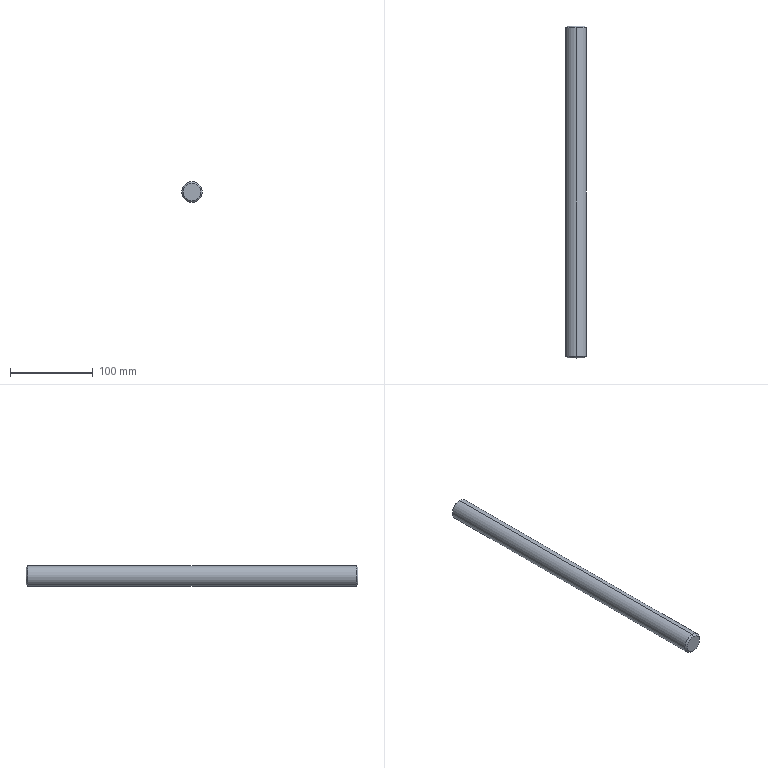Part | STEP file | BCC3 H13_3 | 1 solid | 12 faces | box 25 x 400 x 25 mm | volume 195748 mm3 | cone 6 | cylinder 4 | plane 2 | commonest cylinder face diameters 5 x2 25 x2
STEP:
#1=CARTESIAN_POINT('',(0.,0.,0.));
#2=DIRECTION('',(0.,0.,1.));
#3=DIRECTION('',(1.,0.,0.));
#4=AXIS2_PLACEMENT_3D('',#1,#2,#3);
#5=CARTESIAN_POINT('',(0.,385.,2.5));
#6=VERTEX_POINT('',#5);
#7=CARTESIAN_POINT('',(0.,400.,2.5));
#8=VERTEX_POINT('',#7);
#9=CARTESIAN_POINT('',(0.,400.,2.5));
#10=DIRECTION('',(0.,1.,0.));
#11=VECTOR('',#10,1.);
#12=LINE('',#9,#11);
#13=CARTESIAN_POINT('',(0.,400.,0.));
#14=DIRECTION('',(0.,1.,0.));
#15=DIRECTION('',(0.,0.,1.));
#16=AXIS2_PLACEMENT_3D('',#13,#14,#15);
#17=CYLINDRICAL_SURFACE('',#16,2.5);
#18=CARTESIAN_POINT('',(6.283,0.));
#19=DIRECTION('',(0.,1.));
#20=VECTOR('',#19,1.);
#21=LINE('',#18,#20);
#22=(GEOMETRIC_REPRESENTATION_CONTEXT(2)PARAMETRIC_REPRESENTATION_CONTEXT()REPRESENTATION_CONTEXT('',''));
#23=DEFINITIONAL_REPRESENTATION('',(#21),#22);
#24=PCURVE('',#17,#23);
#25=CARTESIAN_POINT('',(0.,400.,0.));
#26=DIRECTION('',(0.,1.,0.));
#27=DIRECTION('',(0.,0.,1.));
#28=AXIS2_PLACEMENT_3D('',#25,#26,#27);
#29=CYLINDRICAL_SURFACE('',#28,2.5);
#30=CARTESIAN_POINT('',(0.,0.));
#31=DIRECTION('',(0.,1.));
#32=VECTOR('',#31,1.);
#33=LINE('',#30,#32);
#34=(GEOMETRIC_REPRESENTATION_CONTEXT(2)PARAMETRIC_REPRESENTATION_CONTEXT()REPRESENTATION_CONTEXT('',''));
#35=DEFINITIONAL_REPRESENTATION('',(#33),#34);
#36=PCURVE('',#29,#35);
#37=SURFACE_CURVE('',#12,(#24,#36),.PCURVE_S1.);
#38=EDGE_CURVE('',#6,#8,#37,.T.);
#39=ORIENTED_EDGE('',*,*,#38,.T.);
#40=CARTESIAN_POINT('',(0.,400.,-2.5));
#41=VERTEX_POINT('',#40);
#42=CARTESIAN_POINT('',(0.,400.,0.));
#43=DIRECTION('',(0.,1.,0.));
#44=DIRECTION('',(0.,0.,1.));
#45=AXIS2_PLACEMENT_3D('',#42,#43,#44);
#46=CIRCLE('',#45,2.5);
#47=CARTESIAN_POINT('',(0.,0.));
#48=DIRECTION('',(1.,0.));
#49=VECTOR('',#48,1.);
#50=LINE('',#47,#49);
#51=(GEOMETRIC_REPRESENTATION_CONTEXT(2)PARAMETRIC_REPRESENTATION_CONTEXT()REPRESENTATION_CONTEXT('',''));
#52=DEFINITIONAL_REPRESENTATION('',(#50),#51);
#53=PCURVE('',#17,#52);
#54=CARTESIAN_POINT('',(0.,400.,0.));
#55=DIRECTION('',(0.,1.,0.));
#56=DIRECTION('',(0.,0.,1.));
#57=AXIS2_PLACEMENT_3D('',#54,#55,#56);
#58=PLANE('',#57);
#59=CARTESIAN_POINT('',(0.,0.));
#60=DIRECTION('',(1.,0.));
#61=AXIS2_PLACEMENT_2D('',#59,#60);
#62=CIRCLE('',#61,2.5);
#63=(GEOMETRIC_REPRESENTATION_CONTEXT(2)PARAMETRIC_REPRESENTATION_CONTEXT()REPRESENTATION_CONTEXT('',''));
#64=DEFINITIONAL_REPRESENTATION('',(#62),#63);
#65=PCURVE('',#58,#64);
#66=SURFACE_CURVE('',#46,(#53,#65),.PCURVE_S1.);
#67=EDGE_CURVE('',#41,#8,#66,.T.);
#68=ORIENTED_EDGE('',*,*,#67,.F.);
#69=CARTESIAN_POINT('',(0.,385.,-2.5));
#70=VERTEX_POINT('',#69);
#71=CARTESIAN_POINT('',(0.,400.,-2.5));
#72=DIRECTION('',(0.,1.,0.));
#73=VECTOR('',#72,1.);
#74=LINE('',#71,#73);
#75=CARTESIAN_POINT('',(3.142,0.));
#76=DIRECTION('',(0.,1.));
#77=VECTOR('',#76,1.);
#78=LINE('',#75,#77);
#79=(GEOMETRIC_REPRESENTATION_CONTEXT(2)PARAMETRIC_REPRESENTATION_CONTEXT()REPRESENTATION_CONTEXT('',''));
#80=DEFINITIONAL_REPRESENTATION('',(#78),#79);
#81=PCURVE('',#17,#80);
#82=CARTESIAN_POINT('',(3.142,0.));
#83=DIRECTION('',(0.,1.));
#84=VECTOR('',#83,1.);
#85=LINE('',#82,#84);
#86=(GEOMETRIC_REPRESENTATION_CONTEXT(2)PARAMETRIC_REPRESENTATION_CONTEXT()REPRESENTATION_CONTEXT('',''));
#87=DEFINITIONAL_REPRESENTATION('',(#85),#86);
#88=PCURVE('',#29,#87);
#89=SURFACE_CURVE('',#74,(#81,#88),.PCURVE_S1.);
#90=EDGE_CURVE('',#70,#41,#89,.T.);
#91=ORIENTED_EDGE('',*,*,#90,.F.);
#92=CARTESIAN_POINT('',(0.,385.,0.));
#93=DIRECTION('',(0.,1.,0.));
#94=DIRECTION('',(0.,0.,1.));
#95=AXIS2_PLACEMENT_3D('',#92,#93,#94);
#96=CIRCLE('',#95,2.5);
#97=CARTESIAN_POINT('',(0.,-15.));
#98=DIRECTION('',(1.,0.));
#99=VECTOR('',#98,1.);
#100=LINE('',#97,#99);
#101=(GEOMETRIC_REPRESENTATION_CONTEXT(2)PARAMETRIC_REPRESENTATION_CONTEXT()REPRESENTATION_CONTEXT('',''));
#102=DEFINITIONAL_REPRESENTATION('',(#100),#101);
#103=PCURVE('',#17,#102);
#104=CARTESIAN_POINT('',(0.,385.,0.));
#105=DIRECTION('',(0.,1.,0.));
#106=DIRECTION('',(0.,0.,1.));
#107=AXIS2_PLACEMENT_3D('',#104,#105,#106);
#108=CONICAL_SURFACE('',#107,2.5,1.03);
#109=CARTESIAN_POINT('',(0.,0.));
#110=DIRECTION('',(1.,0.));
#111=VECTOR('',#110,1.);
#112=LINE('',#109,#111);
#113=(GEOMETRIC_REPRESENTATION_CONTEXT(2)PARAMETRIC_REPRESENTATION_CONTEXT()REPRESENTATION_CONTEXT('',''));
#114=DEFINITIONAL_REPRESENTATION('',(#112),#113);
#115=PCURVE('',#108,#114);
#116=SURFACE_CURVE('',#96,(#103,#115),.PCURVE_S1.);
#117=EDGE_CURVE('',#70,#6,#116,.T.);
#118=ORIENTED_EDGE('',*,*,#117,.T.);
#119=EDGE_LOOP('',(#39,#68,#91,#118));
#120=FACE_BOUND('',#119,.F.);
#121=ADVANCED_FACE('',(#120),#17,.F.);
#122=ORIENTED_EDGE('',*,*,#117,.F.);
#123=CARTESIAN_POINT('',(0.,383.498,0.));
#124=VERTEX_POINT('',#123);
#125=CARTESIAN_POINT('',(0.,385.,-2.5));
#126=DIRECTION('',(0.,0.515,-0.8572));
#127=VECTOR('',#126,1.);
#128=LINE('',#125,#127);
#129=CARTESIAN_POINT('',(3.142,0.));
#130=DIRECTION('',(0.,1.));
#131=VECTOR('',#130,1.);
#132=LINE('',#129,#131);
#133=(GEOMETRIC_REPRESENTATION_CONTEXT(2)PARAMETRIC_REPRESENTATION_CONTEXT()REPRESENTATION_CONTEXT('',''));
#134=DEFINITIONAL_REPRESENTATION('',(#132),#133);
#135=PCURVE('',#108,#134);
#136=CARTESIAN_POINT('',(0.,385.,0.));
#137=DIRECTION('',(0.,1.,0.));
#138=DIRECTION('',(0.,0.,1.));
#139=AXIS2_PLACEMENT_3D('',#136,#137,#138);
#140=CONICAL_SURFACE('',#139,2.5,1.03);
#141=CARTESIAN_POINT('',(3.142,0.));
#142=DIRECTION('',(0.,1.));
#143=VECTOR('',#142,1.);
#144=LINE('',#141,#143);
#145=(GEOMETRIC_REPRESENTATION_CONTEXT(2)PARAMETRIC_REPRESENTATION_CONTEXT()REPRESENTATION_CONTEXT('',''));
#146=DEFINITIONAL_REPRESENTATION('',(#144),#145);
#147=PCURVE('',#140,#146);
#148=SURFACE_CURVE('',#128,(#135,#147),.PCURVE_S1.);
#149=EDGE_CURVE('',#124,#70,#148,.T.);
#150=ORIENTED_EDGE('',*,*,#149,.F.);
#151=CARTESIAN_POINT('',(0.,385.,2.5));
#152=DIRECTION('',(0.,0.515,0.8572));
#153=VECTOR('',#152,1.);
#154=LINE('',#151,#153);
#155=CARTESIAN_POINT('',(6.283,0.));
#156=DIRECTION('',(0.,1.));
#157=VECTOR('',#156,1.);
#158=LINE('',#155,#157);
#159=(GEOMETRIC_REPRESENTATION_CONTEXT(2)PARAMETRIC_REPRESENTATION_CONTEXT()REPRESENTATION_CONTEXT('',''));
#160=DEFINITIONAL_REPRESENTATION('',(#158),#159);
#161=PCURVE('',#108,#160);
#162=CARTESIAN_POINT('',(0.,0.));
#163=DIRECTION('',(0.,1.));
#164=VECTOR('',#163,1.);
#165=LINE('',#162,#164);
#166=(GEOMETRIC_REPRESENTATION_CONTEXT(2)PARAMETRIC_REPRESENTATION_CONTEXT()REPRESENTATION_CONTEXT('',''));
#167=DEFINITIONAL_REPRESENTATION('',(#165),#166);
#168=PCURVE('',#140,#167);
#169=SURFACE_CURVE('',#154,(#161,#168),.PCURVE_S1.);
#170=EDGE_CURVE('',#124,#6,#169,.T.);
#171=ORIENTED_EDGE('',*,*,#170,.T.);
#172=EDGE_LOOP('',(#122,#150,#171));
#173=FACE_BOUND('',#172,.F.);
#174=ADVANCED_FACE('',(#173),#108,.F.);
#175=CARTESIAN_POINT('',(0.,400.,10.5));
#176=VERTEX_POINT('',#175);
#177=CARTESIAN_POINT('',(0.,400.,-10.5));
#178=VERTEX_POINT('',#177);
#179=CARTESIAN_POINT('',(0.,400.,0.));
#180=DIRECTION('',(0.,1.,0.));
#181=DIRECTION('',(0.,0.,1.));
#182=AXIS2_PLACEMENT_3D('',#179,#180,#181);
#183=CIRCLE('',#182,10.5);
#184=CARTESIAN_POINT('',(0.,400.,0.));
#185=DIRECTION('',(0.,-1.,0.));
#186=DIRECTION('',(0.,0.,-1.));
#187=AXIS2_PLACEMENT_3D('',#184,#185,#186);
#188=CONICAL_SURFACE('',#187,10.5,0.7854);
#189=CARTESIAN_POINT('',(3.142,0.));
#190=DIRECTION('',(-1.,0.));
#191=VECTOR('',#190,1.);
#192=LINE('',#189,#191);
#193=(GEOMETRIC_REPRESENTATION_CONTEXT(2)PARAMETRIC_REPRESENTATION_CONTEXT()REPRESENTATION_CONTEXT('',''));
#194=DEFINITIONAL_REPRESENTATION('',(#192),#193);
#195=PCURVE('',#188,#194);
#196=CARTESIAN_POINT('',(0.,0.));
#197=DIRECTION('',(1.,0.));
#198=AXIS2_PLACEMENT_2D('',#196,#197);
#199=CIRCLE('',#198,10.5);
#200=(GEOMETRIC_REPRESENTATION_CONTEXT(2)PARAMETRIC_REPRESENTATION_CONTEXT()REPRESENTATION_CONTEXT('',''));
#201=DEFINITIONAL_REPRESENTATION('',(#199),#200);
#202=PCURVE('',#58,#201);
#203=SURFACE_CURVE('',#183,(#195,#202),.PCURVE_S1.);
#204=EDGE_CURVE('',#176,#178,#203,.T.);
#205=ORIENTED_EDGE('',*,*,#204,.F.);
#206=CARTESIAN_POINT('',(0.,398.,12.5));
#207=VERTEX_POINT('',#206);
#208=CARTESIAN_POINT('',(0.,400.,10.5));
#209=DIRECTION('',(0.,-0.7071,0.7071));
#210=VECTOR('',#209,1.);
#211=LINE('',#208,#210);
#212=CARTESIAN_POINT('',(3.142,0.));
#213=DIRECTION('',(0.,1.));
#214=VECTOR('',#213,1.);
#215=LINE('',#212,#214);
#216=(GEOMETRIC_REPRESENTATION_CONTEXT(2)PARAMETRIC_REPRESENTATION_CONTEXT()REPRESENTATION_CONTEXT('',''));
#217=DEFINITIONAL_REPRESENTATION('',(#215),#216);
#218=PCURVE('',#188,#217);
#219=CARTESIAN_POINT('',(0.,400.,0.));
#220=DIRECTION('',(0.,-1.,0.));
#221=DIRECTION('',(0.,0.,-1.));
#222=AXIS2_PLACEMENT_3D('',#219,#220,#221);
#223=CONICAL_SURFACE('',#222,10.5,0.7854);
#224=CARTESIAN_POINT('',(3.142,0.));
#225=DIRECTION('',(0.,1.));
#226=VECTOR('',#225,1.);
#227=LINE('',#224,#226);
#228=(GEOMETRIC_REPRESENTATION_CONTEXT(2)PARAMETRIC_REPRESENTATION_CONTEXT()REPRESENTATION_CONTEXT('',''));
#229=DEFINITIONAL_REPRESENTATION('',(#227),#228);
#230=PCURVE('',#223,#229);
#231=SURFACE_CURVE('',#211,(#218,#230),.PCURVE_S1.);
#232=EDGE_CURVE('',#176,#207,#231,.T.);
#233=ORIENTED_EDGE('',*,*,#232,.T.);
#234=CARTESIAN_POINT('',(0.,398.,-12.5));
#235=VERTEX_POINT('',#234);
#236=CARTESIAN_POINT('',(0.,398.,0.));
#237=DIRECTION('',(0.,-1.,0.));
#238=DIRECTION('',(0.,0.,1.));
#239=AXIS2_PLACEMENT_3D('',#236,#237,#238);
#240=CIRCLE('',#239,12.5);
#241=CARTESIAN_POINT('',(-3.142,2.));
#242=DIRECTION('',(1.,0.));
#243=VECTOR('',#242,1.);
#244=LINE('',#241,#243);
#245=(GEOMETRIC_REPRESENTATION_CONTEXT(2)PARAMETRIC_REPRESENTATION_CONTEXT()REPRESENTATION_CONTEXT('',''));
#246=DEFINITIONAL_REPRESENTATION('',(#244),#245);
#247=PCURVE('',#188,#246);
#248=CARTESIAN_POINT('',(0.,400.,0.));
#249=DIRECTION('',(0.,-1.,0.));
#250=DIRECTION('',(0.,0.,-1.));
#251=AXIS2_PLACEMENT_3D('',#248,#249,#250);
#252=CYLINDRICAL_SURFACE('',#251,12.5);
#253=CARTESIAN_POINT('',(-3.142,2.));
#254=DIRECTION('',(1.,0.));
#255=VECTOR('',#254,1.);
#256=LINE('',#253,#255);
#257=(GEOMETRIC_REPRESENTATION_CONTEXT(2)PARAMETRIC_REPRESENTATION_CONTEXT()REPRESENTATION_CONTEXT('',''));
#258=DEFINITIONAL_REPRESENTATION('',(#256),#257);
#259=PCURVE('',#252,#258);
#260=SURFACE_CURVE('',#240,(#247,#259),.PCURVE_S1.);
#261=EDGE_CURVE('',#235,#207,#260,.T.);
#262=ORIENTED_EDGE('',*,*,#261,.F.);
#263=CARTESIAN_POINT('',(0.,400.,-10.5));
#264=DIRECTION('',(0.,-0.7071,-0.7071));
#265=VECTOR('',#264,1.);
#266=LINE('',#263,#265);
#267=CARTESIAN_POINT('',(0.,0.));
#268=DIRECTION('',(0.,1.));
#269=VECTOR('',#268,1.);
#270=LINE('',#267,#269);
#271=(GEOMETRIC_REPRESENTATION_CONTEXT(2)PARAMETRIC_REPRESENTATION_CONTEXT()REPRESENTATION_CONTEXT('',''));
#272=DEFINITIONAL_REPRESENTATION('',(#270),#271);
#273=PCURVE('',#188,#272);
#274=CARTESIAN_POINT('',(6.283,0.));
#275=DIRECTION('',(0.,1.));
#276=VECTOR('',#275,1.);
#277=LINE('',#274,#276);
#278=(GEOMETRIC_REPRESENTATION_CONTEXT(2)PARAMETRIC_REPRESENTATION_CONTEXT()REPRESENTATION_CONTEXT('',''));
#279=DEFINITIONAL_REPRESENTATION('',(#277),#278);
#280=PCURVE('',#223,#279);
#281=SURFACE_CURVE('',#266,(#273,#280),.PCURVE_S1.);
#282=EDGE_CURVE('',#178,#235,#281,.T.);
#283=ORIENTED_EDGE('',*,*,#282,.F.);
#284=EDGE_LOOP('',(#205,#233,#262,#283));
#285=FACE_BOUND('',#284,.T.);
#286=ADVANCED_FACE('',(#285),#188,.T.);
#287=CARTESIAN_POINT('',(0.,0.,-10.5));
#288=VERTEX_POINT('',#287);
#289=CARTESIAN_POINT('',(0.,0.,10.5));
#290=VERTEX_POINT('',#289);
#291=CARTESIAN_POINT('',(0.,0.,0.));
#292=DIRECTION('',(0.,-1.,0.));
#293=DIRECTION('',(0.,0.,1.));
#294=AXIS2_PLACEMENT_3D('',#291,#292,#293);
#295=CIRCLE('',#294,10.5);
#296=CARTESIAN_POINT('',(0.,2.,0.));
#297=DIRECTION('',(0.,1.,0.));
#298=DIRECTION('',(0.,0.,1.));
#299=AXIS2_PLACEMENT_3D('',#296,#297,#298);
#300=CONICAL_SURFACE('',#299,12.5,0.7854);
#301=CARTESIAN_POINT('',(6.283,-2.));
#302=DIRECTION('',(-1.,0.));
#303=VECTOR('',#302,1.);
#304=LINE('',#301,#303);
#305=(GEOMETRIC_REPRESENTATION_CONTEXT(2)PARAMETRIC_REPRESENTATION_CONTEXT()REPRESENTATION_CONTEXT('',''));
#306=DEFINITIONAL_REPRESENTATION('',(#304),#305);
#307=PCURVE('',#300,#306);
#308=CARTESIAN_POINT('',(0.,0.,0.));
#309=DIRECTION('',(0.,1.,0.));
#310=DIRECTION('',(0.,0.,1.));
#311=AXIS2_PLACEMENT_3D('',#308,#309,#310);
#312=PLANE('',#311);
#313=CARTESIAN_POINT('',(10.5,0.));
#314=CARTESIAN_POINT('',(10.5,-18.187));
#315=CARTESIAN_POINT('',(-5.25,-9.093));
#316=CARTESIAN_POINT('',(-21.,0.));
#317=CARTESIAN_POINT('',(-5.25,9.093));
#318=CARTESIAN_POINT('',(10.5,18.187));
#319=CARTESIAN_POINT('',(10.5,0.));
#320=(BOUNDED_CURVE()B_SPLINE_CURVE(2,(#313,#314,#315,#316,#317,#318,#319),.UNSPECIFIED.,.T.,.F.)B_SPLINE_CURVE_WITH_KNOTS((1,2,2,2,2,1),(-2.094,0.,2.094,4.189,6.283,8.378),.UNSPECIFIED.)CURVE()GEOMETRIC_REPRESENTATION_ITEM()RATIONAL_B_SPLINE_CURVE((1.,0.5,1.,0.5,1.,0.5,1.))REPRESENTATION_ITEM(''));
#321=(GEOMETRIC_REPRESENTATION_CONTEXT(2)PARAMETRIC_REPRESENTATION_CONTEXT()REPRESENTATION_CONTEXT('',''));
#322=DEFINITIONAL_REPRESENTATION('',(#320),#321);
#323=PCURVE('',#312,#322);
#324=SURFACE_CURVE('',#295,(#307,#323),.PCURVE_S1.);
#325=EDGE_CURVE('',#288,#290,#324,.T.);
#326=ORIENTED_EDGE('',*,*,#325,.F.);
#327=CARTESIAN_POINT('',(0.,2.,-12.5));
#328=VERTEX_POINT('',#327);
#329=CARTESIAN_POINT('',(0.,2.,-12.5));
#330=DIRECTION('',(0.,0.7071,-0.7071));
#331=VECTOR('',#330,1.);
#332=LINE('',#329,#331);
#333=CARTESIAN_POINT('',(3.142,0.));
#334=DIRECTION('',(0.,1.));
#335=VECTOR('',#334,1.);
#336=LINE('',#333,#335);
#337=(GEOMETRIC_REPRESENTATION_CONTEXT(2)PARAMETRIC_REPRESENTATION_CONTEXT()REPRESENTATION_CONTEXT('',''));
#338=DEFINITIONAL_REPRESENTATION('',(#336),#337);
#339=PCURVE('',#300,#338);
#340=CARTESIAN_POINT('',(0.,2.,0.));
#341=DIRECTION('',(0.,1.,0.));
#342=DIRECTION('',(0.,0.,1.));
#343=AXIS2_PLACEMENT_3D('',#340,#341,#342);
#344=CONICAL_SURFACE('',#343,12.5,0.7854);
#345=CARTESIAN_POINT('',(3.142,0.));
#346=DIRECTION('',(0.,1.));
#347=VECTOR('',#346,1.);
#348=LINE('',#345,#347);
#349=(GEOMETRIC_REPRESENTATION_CONTEXT(2)PARAMETRIC_REPRESENTATION_CONTEXT()REPRESENTATION_CONTEXT('',''));
#350=DEFINITIONAL_REPRESENTATION('',(#348),#349);
#351=PCURVE('',#344,#350);
#352=SURFACE_CURVE('',#332,(#339,#351),.PCURVE_S1.);
#353=EDGE_CURVE('',#288,#328,#352,.T.);
#354=ORIENTED_EDGE('',*,*,#353,.T.);
#355=CARTESIAN_POINT('',(0.,2.,12.5));
#356=VERTEX_POINT('',#355);
#357=CARTESIAN_POINT('',(0.,2.,0.));
#358=DIRECTION('',(0.,1.,0.));
#359=DIRECTION('',(0.,0.,1.));
#360=AXIS2_PLACEMENT_3D('',#357,#358,#359);
#361=CIRCLE('',#360,12.5);
#362=CARTESIAN_POINT('',(0.,0.));
#363=DIRECTION('',(1.,0.));
#364=VECTOR('',#363,1.);
#365=LINE('',#362,#364);
#366=(GEOMETRIC_REPRESENTATION_CONTEXT(2)PARAMETRIC_REPRESENTATION_CONTEXT()REPRESENTATION_CONTEXT('',''));
#367=DEFINITIONAL_REPRESENTATION('',(#365),#366);
#368=PCURVE('',#300,#367);
#369=CARTESIAN_POINT('',(3.142,398.));
#370=DIRECTION('',(-1.,0.));
#371=VECTOR('',#370,1.);
#372=LINE('',#369,#371);
#373=(GEOMETRIC_REPRESENTATION_CONTEXT(2)PARAMETRIC_REPRESENTATION_CONTEXT()REPRESENTATION_CONTEXT('',''));
#374=DEFINITIONAL_REPRESENTATION('',(#372),#373);
#375=PCURVE('',#252,#374);
#376=SURFACE_CURVE('',#361,(#368,#375),.PCURVE_S1.);
#377=EDGE_CURVE('',#356,#328,#376,.T.);
#378=ORIENTED_EDGE('',*,*,#377,.F.);
#379=CARTESIAN_POINT('',(0.,2.,12.5));
#380=DIRECTION('',(0.,0.7071,0.7071));
#381=VECTOR('',#380,1.);
#382=LINE('',#379,#381);
#383=CARTESIAN_POINT('',(0.,0.));
#384=DIRECTION('',(0.,1.));
#385=VECTOR('',#384,1.);
#386=LINE('',#383,#385);
#387=(GEOMETRIC_REPRESENTATION_CONTEXT(2)PARAMETRIC_REPRESENTATION_CONTEXT()REPRESENTATION_CONTEXT('',''));
#388=DEFINITIONAL_REPRESENTATION('',(#386),#387);
#389=PCURVE('',#300,#388);
#390=CARTESIAN_POINT('',(6.283,0.));
#391=DIRECTION('',(0.,1.));
#392=VECTOR('',#391,1.);
#393=LINE('',#390,#392);
#394=(GEOMETRIC_REPRESENTATION_CONTEXT(2)PARAMETRIC_REPRESENTATION_CONTEXT()REPRESENTATION_CONTEXT('',''));
#395=DEFINITIONAL_REPRESENTATION('',(#393),#394);
#396=PCURVE('',#344,#395);
#397=SURFACE_CURVE('',#382,(#389,#396),.PCURVE_S1.);
#398=EDGE_CURVE('',#290,#356,#397,.T.);
#399=ORIENTED_EDGE('',*,*,#398,.F.);
#400=EDGE_LOOP('',(#326,#354,#378,#399));
#401=FACE_BOUND('',#400,.T.);
#402=ADVANCED_FACE('',(#401),#300,.T.);
#403=ORIENTED_EDGE('',*,*,#261,.T.);
#404=CARTESIAN_POINT('',(0.,400.,12.5));
#405=DIRECTION('',(0.,-1.,0.));
#406=VECTOR('',#405,1.);
#407=LINE('',#404,#406);
#408=CARTESIAN_POINT('',(3.142,0.));
#409=DIRECTION('',(0.,1.));
#410=VECTOR('',#409,1.);
#411=LINE('',#408,#410);
#412=(GEOMETRIC_REPRESENTATION_CONTEXT(2)PARAMETRIC_REPRESENTATION_CONTEXT()REPRESENTATION_CONTEXT('',''));
#413=DEFINITIONAL_REPRESENTATION('',(#411),#412);
#414=PCURVE('',#252,#413);
#415=CARTESIAN_POINT('',(0.,400.,0.));
#416=DIRECTION('',(0.,-1.,0.));
#417=DIRECTION('',(0.,0.,-1.));
#418=AXIS2_PLACEMENT_3D('',#415,#416,#417);
#419=CYLINDRICAL_SURFACE('',#418,12.5);
#420=CARTESIAN_POINT('',(3.142,0.));
#421=DIRECTION('',(0.,1.));
#422=VECTOR('',#421,1.);
#423=LINE('',#420,#422);
#424=(GEOMETRIC_REPRESENTATION_CONTEXT(2)PARAMETRIC_REPRESENTATION_CONTEXT()REPRESENTATION_CONTEXT('',''));
#425=DEFINITIONAL_REPRESENTATION('',(#423),#424);
#426=PCURVE('',#419,#425);
#427=SURFACE_CURVE('',#407,(#414,#426),.PCURVE_S1.);
#428=EDGE_CURVE('',#207,#356,#427,.T.);
#429=ORIENTED_EDGE('',*,*,#428,.T.);
#430=ORIENTED_EDGE('',*,*,#377,.T.);
#431=CARTESIAN_POINT('',(0.,400.,-12.5));
#432=DIRECTION('',(0.,-1.,0.));
#433=VECTOR('',#432,1.);
#434=LINE('',#431,#433);
#435=CARTESIAN_POINT('',(0.,0.));
#436=DIRECTION('',(0.,1.));
#437=VECTOR('',#436,1.);
#438=LINE('',#435,#437);
#439=(GEOMETRIC_REPRESENTATION_CONTEXT(2)PARAMETRIC_REPRESENTATION_CONTEXT()REPRESENTATION_CONTEXT('',''));
#440=DEFINITIONAL_REPRESENTATION('',(#438),#439);
#441=PCURVE('',#252,#440);
#442=CARTESIAN_POINT('',(6.283,0.));
#443=DIRECTION('',(0.,1.));
#444=VECTOR('',#443,1.);
#445=LINE('',#442,#444);
#446=(GEOMETRIC_REPRESENTATION_CONTEXT(2)PARAMETRIC_REPRESENTATION_CONTEXT()REPRESENTATION_CONTEXT('',''));
#447=DEFINITIONAL_REPRESENTATION('',(#445),#446);
#448=PCURVE('',#419,#447);
#449=SURFACE_CURVE('',#434,(#441,#448),.PCURVE_S1.);
#450=EDGE_CURVE('',#235,#328,#449,.T.);
#451=ORIENTED_EDGE('',*,*,#450,.F.);
#452=EDGE_LOOP('',(#403,#429,#430,#451));
#453=FACE_BOUND('',#452,.T.);
#454=ADVANCED_FACE('',(#453),#252,.T.);
#455=ORIENTED_EDGE('',*,*,#428,.F.);
#456=CARTESIAN_POINT('',(0.,398.,0.));
#457=DIRECTION('',(0.,-1.,0.));
#458=DIRECTION('',(0.,0.,1.));
#459=AXIS2_PLACEMENT_3D('',#456,#457,#458);
#460=CIRCLE('',#459,12.5);
#461=CARTESIAN_POINT('',(3.142,2.));
#462=DIRECTION('',(1.,0.));
#463=VECTOR('',#462,1.);
#464=LINE('',#461,#463);
#465=(GEOMETRIC_REPRESENTATION_CONTEXT(2)PARAMETRIC_REPRESENTATION_CONTEXT()REPRESENTATION_CONTEXT('',''));
#466=DEFINITIONAL_REPRESENTATION('',(#464),#465);
#467=PCURVE('',#419,#466);
#468=CARTESIAN_POINT('',(3.142,2.));
#469=DIRECTION('',(1.,0.));
#470=VECTOR('',#469,1.);
#471=LINE('',#468,#470);
#472=(GEOMETRIC_REPRESENTATION_CONTEXT(2)PARAMETRIC_REPRESENTATION_CONTEXT()REPRESENTATION_CONTEXT('',''));
#473=DEFINITIONAL_REPRESENTATION('',(#471),#472);
#474=PCURVE('',#223,#473);
#475=SURFACE_CURVE('',#460,(#467,#474),.PCURVE_S1.);
#476=EDGE_CURVE('',#207,#235,#475,.T.);
#477=ORIENTED_EDGE('',*,*,#476,.T.);
#478=ORIENTED_EDGE('',*,*,#450,.T.);
#479=CARTESIAN_POINT('',(0.,2.,0.));
#480=DIRECTION('',(0.,1.,0.));
#481=DIRECTION('',(0.,0.,1.));
#482=AXIS2_PLACEMENT_3D('',#479,#480,#481);
#483=CIRCLE('',#482,12.5);
#484=CARTESIAN_POINT('',(9.425,398.));
#485=DIRECTION('',(-1.,0.));
#486=VECTOR('',#485,1.);
#487=LINE('',#484,#486);
#488=(GEOMETRIC_REPRESENTATION_CONTEXT(2)PARAMETRIC_REPRESENTATION_CONTEXT()REPRESENTATION_CONTEXT('',''));
#489=DEFINITIONAL_REPRESENTATION('',(#487),#488);
#490=PCURVE('',#419,#489);
#491=CARTESIAN_POINT('',(0.,0.));
#492=DIRECTION('',(1.,0.));
#493=VECTOR('',#492,1.);
#494=LINE('',#491,#493);
#495=(GEOMETRIC_REPRESENTATION_CONTEXT(2)PARAMETRIC_REPRESENTATION_CONTEXT()REPRESENTATION_CONTEXT('',''));
#496=DEFINITIONAL_REPRESENTATION('',(#494),#495);
#497=PCURVE('',#344,#496);
#498=SURFACE_CURVE('',#483,(#490,#497),.PCURVE_S1.);
#499=EDGE_CURVE('',#328,#356,#498,.T.);
#500=ORIENTED_EDGE('',*,*,#499,.T.);
#501=EDGE_LOOP('',(#455,#477,#478,#500));
#502=FACE_BOUND('',#501,.T.);
#503=ADVANCED_FACE('',(#502),#419,.T.);
#504=CARTESIAN_POINT('',(0.,400.,0.));
#505=DIRECTION('',(0.,1.,0.));
#506=DIRECTION('',(0.,0.,1.));
#507=AXIS2_PLACEMENT_3D('',#504,#505,#506);
#508=CIRCLE('',#507,2.5);
#509=CARTESIAN_POINT('',(0.,0.));
#510=DIRECTION('',(1.,0.));
#511=AXIS2_PLACEMENT_2D('',#509,#510);
#512=CIRCLE('',#511,2.5);
#513=(GEOMETRIC_REPRESENTATION_CONTEXT(2)PARAMETRIC_REPRESENTATION_CONTEXT()REPRESENTATION_CONTEXT('',''));
#514=DEFINITIONAL_REPRESENTATION('',(#512),#513);
#515=PCURVE('',#58,#514);
#516=CARTESIAN_POINT('',(0.,0.));
#517=DIRECTION('',(1.,0.));
#518=VECTOR('',#517,1.);
#519=LINE('',#516,#518);
#520=(GEOMETRIC_REPRESENTATION_CONTEXT(2)PARAMETRIC_REPRESENTATION_CONTEXT()REPRESENTATION_CONTEXT('',''));
#521=DEFINITIONAL_REPRESENTATION('',(#519),#520);
#522=PCURVE('',#29,#521);
#523=SURFACE_CURVE('',#508,(#515,#522),.PCURVE_S1.);
#524=EDGE_CURVE('',#8,#41,#523,.T.);
#525=ORIENTED_EDGE('',*,*,#524,.F.);
#526=ORIENTED_EDGE('',*,*,#67,.F.);
#527=EDGE_LOOP('',(#525,#526));
#528=FACE_BOUND('',#527,.T.);
#529=CARTESIAN_POINT('',(0.,400.,0.));
#530=DIRECTION('',(0.,1.,0.));
#531=DIRECTION('',(0.,0.,1.));
#532=AXIS2_PLACEMENT_3D('',#529,#530,#531);
#533=CIRCLE('',#532,10.5);
#534=CARTESIAN_POINT('',(0.,0.));
#535=DIRECTION('',(1.,0.));
#536=AXIS2_PLACEMENT_2D('',#534,#535);
#537=CIRCLE('',#536,10.5);
#538=(GEOMETRIC_REPRESENTATION_CONTEXT(2)PARAMETRIC_REPRESENTATION_CONTEXT()REPRESENTATION_CONTEXT('',''));
#539=DEFINITIONAL_REPRESENTATION('',(#537),#538);
#540=PCURVE('',#58,#539);
#541=CARTESIAN_POINT('',(9.425,0.));
#542=DIRECTION('',(-1.,0.));
#543=VECTOR('',#542,1.);
#544=LINE('',#541,#543);
#545=(GEOMETRIC_REPRESENTATION_CONTEXT(2)PARAMETRIC_REPRESENTATION_CONTEXT()REPRESENTATION_CONTEXT('',''));
#546=DEFINITIONAL_REPRESENTATION('',(#544),#545);
#547=PCURVE('',#223,#546);
#548=SURFACE_CURVE('',#533,(#540,#547),.PCURVE_S1.);
#549=EDGE_CURVE('',#178,#176,#548,.T.);
#550=ORIENTED_EDGE('',*,*,#549,.T.);
#551=ORIENTED_EDGE('',*,*,#204,.T.);
#552=EDGE_LOOP('',(#550,#551));
#553=FACE_BOUND('',#552,.T.);
#554=ADVANCED_FACE('',(#528,#553),#58,.T.);
#555=CARTESIAN_POINT('',(0.,0.,0.));
#556=DIRECTION('',(0.,-1.,0.));
#557=DIRECTION('',(0.,0.,1.));
#558=AXIS2_PLACEMENT_3D('',#555,#556,#557);
#559=CIRCLE('',#558,10.5);
#560=CARTESIAN_POINT('',(10.5,0.));
#561=CARTESIAN_POINT('',(10.5,-18.187));
#562=CARTESIAN_POINT('',(-5.25,-9.093));
#563=CARTESIAN_POINT('',(-21.,0.));
#564=CARTESIAN_POINT('',(-5.25,9.093));
#565=CARTESIAN_POINT('',(10.5,18.187));
#566=CARTESIAN_POINT('',(10.5,0.));
#567=(BOUNDED_CURVE()B_SPLINE_CURVE(2,(#560,#561,#562,#563,#564,#565,#566),.UNSPECIFIED.,.T.,.F.)B_SPLINE_CURVE_WITH_KNOTS((1,2,2,2,2,1),(-2.094,0.,2.094,4.189,6.283,8.378),.UNSPECIFIED.)CURVE()GEOMETRIC_REPRESENTATION_ITEM()RATIONAL_B_SPLINE_CURVE((1.,0.5,1.,0.5,1.,0.5,1.))REPRESENTATION_ITEM(''));
#568=(GEOMETRIC_REPRESENTATION_CONTEXT(2)PARAMETRIC_REPRESENTATION_CONTEXT()REPRESENTATION_CONTEXT('',''));
#569=DEFINITIONAL_REPRESENTATION('',(#567),#568);
#570=PCURVE('',#312,#569);
#571=CARTESIAN_POINT('',(6.283,-2.));
#572=DIRECTION('',(-1.,0.));
#573=VECTOR('',#572,1.);
#574=LINE('',#571,#573);
#575=(GEOMETRIC_REPRESENTATION_CONTEXT(2)PARAMETRIC_REPRESENTATION_CONTEXT()REPRESENTATION_CONTEXT('',''));
#576=DEFINITIONAL_REPRESENTATION('',(#574),#575);
#577=PCURVE('',#344,#576);
#578=SURFACE_CURVE('',#559,(#570,#577),.PCURVE_S1.);
#579=EDGE_CURVE('',#290,#288,#578,.T.);
#580=ORIENTED_EDGE('',*,*,#579,.T.);
#581=ORIENTED_EDGE('',*,*,#325,.T.);
#582=EDGE_LOOP('',(#580,#581));
#583=FACE_BOUND('',#582,.T.);
#584=ADVANCED_FACE('',(#583),#312,.F.);
#585=ORIENTED_EDGE('',*,*,#353,.F.);
#586=ORIENTED_EDGE('',*,*,#579,.F.);
#587=ORIENTED_EDGE('',*,*,#398,.T.);
#588=ORIENTED_EDGE('',*,*,#499,.F.);
#589=EDGE_LOOP('',(#585,#586,#587,#588));
#590=FACE_BOUND('',#589,.T.);
#591=ADVANCED_FACE('',(#590),#344,.T.);
#592=ORIENTED_EDGE('',*,*,#232,.F.);
#593=ORIENTED_EDGE('',*,*,#549,.F.);
#594=ORIENTED_EDGE('',*,*,#282,.T.);
#595=ORIENTED_EDGE('',*,*,#476,.F.);
#596=EDGE_LOOP('',(#592,#593,#594,#595));
#597=FACE_BOUND('',#596,.T.);
#598=ADVANCED_FACE('',(#597),#223,.T.);
#599=CARTESIAN_POINT('',(0.,385.,0.));
#600=DIRECTION('',(0.,1.,0.));
#601=DIRECTION('',(0.,0.,1.));
#602=AXIS2_PLACEMENT_3D('',#599,#600,#601);
#603=CIRCLE('',#602,2.5);
#604=CARTESIAN_POINT('',(0.,0.));
#605=DIRECTION('',(1.,0.));
#606=VECTOR('',#605,1.);
#607=LINE('',#604,#606);
#608=(GEOMETRIC_REPRESENTATION_CONTEXT(2)PARAMETRIC_REPRESENTATION_CONTEXT()REPRESENTATION_CONTEXT('',''));
#609=DEFINITIONAL_REPRESENTATION('',(#607),#608);
#610=PCURVE('',#140,#609);
#611=CARTESIAN_POINT('',(0.,-15.));
#612=DIRECTION('',(1.,0.));
#613=VECTOR('',#612,1.);
#614=LINE('',#611,#613);
#615=(GEOMETRIC_REPRESENTATION_CONTEXT(2)PARAMETRIC_REPRESENTATION_CONTEXT()REPRESENTATION_CONTEXT('',''));
#616=DEFINITIONAL_REPRESENTATION('',(#614),#615);
#617=PCURVE('',#29,#616);
#618=SURFACE_CURVE('',#603,(#610,#617),.PCURVE_S1.);
#619=EDGE_CURVE('',#6,#70,#618,.T.);
#620=ORIENTED_EDGE('',*,*,#619,.F.);
#621=ORIENTED_EDGE('',*,*,#170,.F.);
#622=ORIENTED_EDGE('',*,*,#149,.T.);
#623=EDGE_LOOP('',(#620,#621,#622));
#624=FACE_BOUND('',#623,.F.);
#625=ADVANCED_FACE('',(#624),#140,.F.);
#626=ORIENTED_EDGE('',*,*,#524,.F.);
#627=ORIENTED_EDGE('',*,*,#38,.F.);
#628=ORIENTED_EDGE('',*,*,#619,.T.);
#629=ORIENTED_EDGE('',*,*,#90,.T.);
#630=EDGE_LOOP('',(#626,#627,#628,#629));
#631=FACE_BOUND('',#630,.F.);
#632=ADVANCED_FACE('',(#631),#29,.F.);
#633=CLOSED_SHELL('',(#121,#174,#286,#402,#454,#503,#554,#584,#591,#598,#625,#632));
#634=MANIFOLD_SOLID_BREP('',#633);
#635=(LENGTH_UNIT()NAMED_UNIT(*)SI_UNIT(.MILLI.,.METRE.));
#636=UNCERTAINTY_MEASURE_WITH_UNIT(LENGTH_MEASURE(0.0000001),#635,'','');
#637=(NAMED_UNIT(*)PLANE_ANGLE_UNIT()SI_UNIT($,.RADIAN.));
#638=(NAMED_UNIT(*)SI_UNIT($,.STERADIAN.)SOLID_ANGLE_UNIT());
#639=(GEOMETRIC_REPRESENTATION_CONTEXT(3)GLOBAL_UNCERTAINTY_ASSIGNED_CONTEXT((#636))GLOBAL_UNIT_ASSIGNED_CONTEXT((#635,#637,#638))REPRESENTATION_CONTEXT('',''));
#640=ADVANCED_BREP_SHAPE_REPRESENTATION('',(#4,#634),#639);